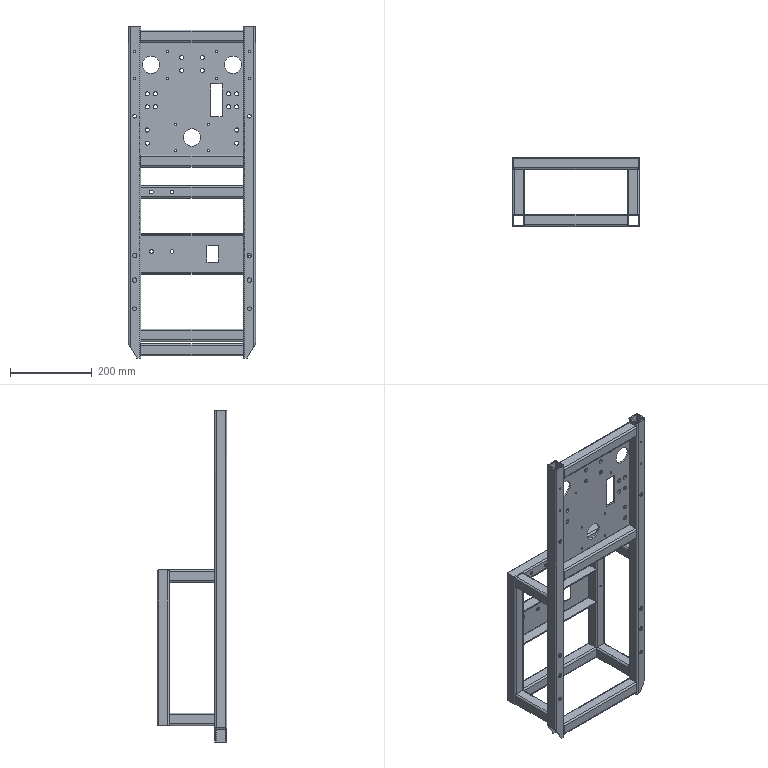Part | NX | features BREP 1, DATUM_CSYS 1, EXTRACT_DATUM_PLANE 1, SKETCH 1 | 1 solid | 415 faces | box 310 x 170 x 810 mm | volume 1667503 mm3 | cylinder 230 | plane 185 | commonest cylinder face diameters 2 x54 8 x54 5 x40 10 x32 9 x28 11 x16